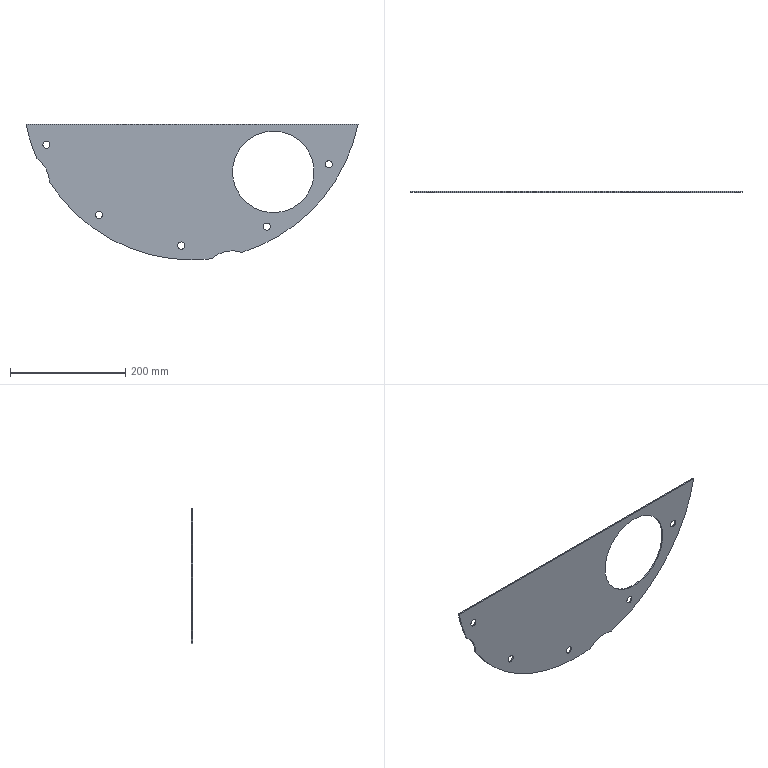Part | SolidWorks | features BaseBody 1 | 1 solid | 22 faces | box 577 x 2 x 236 mm | volume 170029 mm3 | cylinder 19 | plane 3 | commonest cylinder face diameters 12.5 x10 588.679 x4 106 x3 142 x2
STEP:
#1=CARTESIAN_POINT('',(237.632,2.,-121.934));
#2=VERTEX_POINT('',#1);
#3=CARTESIAN_POINT('',(237.632,2.,-134.434));
#4=VERTEX_POINT('',#3);
#5=CARTESIAN_POINT('',(237.632,2.,-128.184));
#6=DIRECTION('',(0.,-1.,0.));
#7=DIRECTION('',(0.,0.,-1.));
#8=AXIS2_PLACEMENT_3D('',#5,#6,#7);
#9=CIRCLE('',#8,6.25);
#10=EDGE_CURVE('',#2,#4,#9,.T.);
#11=ORIENTED_EDGE('',*,*,#10,.F.);
#12=CARTESIAN_POINT('',(237.632,0.,-121.934));
#13=VERTEX_POINT('',#12);
#14=CARTESIAN_POINT('',(237.632,2.,-121.934));
#15=DIRECTION('',(0.,-1.,0.));
#16=VECTOR('',#15,1000.);
#17=LINE('',#14,#16);
#18=EDGE_CURVE('',#2,#13,#17,.T.);
#19=ORIENTED_EDGE('',*,*,#18,.T.);
#20=CARTESIAN_POINT('',(237.632,0.,-134.434));
#21=VERTEX_POINT('',#20);
#22=CARTESIAN_POINT('',(237.632,0.,-128.184));
#23=DIRECTION('',(0.,1.,0.));
#24=DIRECTION('',(0.,0.,-1.));
#25=AXIS2_PLACEMENT_3D('',#22,#23,#24);
#26=CIRCLE('',#25,6.25);
#27=EDGE_CURVE('',#21,#13,#26,.T.);
#28=ORIENTED_EDGE('',*,*,#27,.F.);
#29=CARTESIAN_POINT('',(237.632,2.,-134.434));
#30=DIRECTION('',(0.,-1.,0.));
#31=VECTOR('',#30,1000.);
#32=LINE('',#29,#31);
#33=EDGE_CURVE('',#4,#21,#32,.T.);
#34=ORIENTED_EDGE('',*,*,#33,.F.);
#35=EDGE_LOOP('',(#11,#19,#28,#34));
#36=FACE_OUTER_BOUND('',#35,.T.);
#37=CARTESIAN_POINT('',(237.632,2.,-128.184));
#38=DIRECTION('',(0.,-1.,0.));
#39=DIRECTION('',(0.,0.,-1.));
#40=AXIS2_PLACEMENT_3D('',#37,#38,#39);
#41=CYLINDRICAL_SURFACE('',#40,6.25);
#42=ADVANCED_FACE('',(#36),#41,.F.);
#43=CARTESIAN_POINT('',(-18.702,2.,-263.101));
#44=VERTEX_POINT('',#43);
#45=CARTESIAN_POINT('',(-18.702,2.,-275.601));
#46=VERTEX_POINT('',#45);
#47=CARTESIAN_POINT('',(-18.702,2.,-269.351));
#48=DIRECTION('',(0.,-1.,0.));
#49=DIRECTION('',(0.,0.,-1.));
#50=AXIS2_PLACEMENT_3D('',#47,#48,#49);
#51=CIRCLE('',#50,6.25);
#52=EDGE_CURVE('',#44,#46,#51,.T.);
#53=ORIENTED_EDGE('',*,*,#52,.F.);
#54=CARTESIAN_POINT('',(-18.702,0.,-263.101));
#55=VERTEX_POINT('',#54);
#56=CARTESIAN_POINT('',(-18.702,2.,-263.101));
#57=DIRECTION('',(0.,-1.,0.));
#58=VECTOR('',#57,1000.);
#59=LINE('',#56,#58);
#60=EDGE_CURVE('',#44,#55,#59,.T.);
#61=ORIENTED_EDGE('',*,*,#60,.T.);
#62=CARTESIAN_POINT('',(-18.702,0.,-275.601));
#63=VERTEX_POINT('',#62);
#64=CARTESIAN_POINT('',(-18.702,0.,-269.351));
#65=DIRECTION('',(0.,1.,0.));
#66=DIRECTION('',(0.,0.,-1.));
#67=AXIS2_PLACEMENT_3D('',#64,#65,#66);
#68=CIRCLE('',#67,6.25);
#69=EDGE_CURVE('',#63,#55,#68,.T.);
#70=ORIENTED_EDGE('',*,*,#69,.F.);
#71=CARTESIAN_POINT('',(-18.702,2.,-275.601));
#72=DIRECTION('',(0.,-1.,0.));
#73=VECTOR('',#72,1000.);
#74=LINE('',#71,#73);
#75=EDGE_CURVE('',#46,#63,#74,.T.);
#76=ORIENTED_EDGE('',*,*,#75,.F.);
#77=EDGE_LOOP('',(#53,#61,#70,#76));
#78=FACE_OUTER_BOUND('',#77,.T.);
#79=CARTESIAN_POINT('',(-18.702,2.,-269.351));
#80=DIRECTION('',(0.,-1.,0.));
#81=DIRECTION('',(0.,0.,-1.));
#82=AXIS2_PLACEMENT_3D('',#79,#80,#81);
#83=CYLINDRICAL_SURFACE('',#82,6.25);
#84=ADVANCED_FACE('',(#78),#83,.F.);
#85=CARTESIAN_POINT('',(-253.067,2.,-87.863));
#86=VERTEX_POINT('',#85);
#87=CARTESIAN_POINT('',(-253.067,2.,-100.363));
#88=VERTEX_POINT('',#87);
#89=CARTESIAN_POINT('',(-253.067,2.,-94.113));
#90=DIRECTION('',(0.,-1.,0.));
#91=DIRECTION('',(0.,0.,-1.));
#92=AXIS2_PLACEMENT_3D('',#89,#90,#91);
#93=CIRCLE('',#92,6.25);
#94=EDGE_CURVE('',#86,#88,#93,.T.);
#95=ORIENTED_EDGE('',*,*,#94,.F.);
#96=CARTESIAN_POINT('',(-253.067,0.,-87.863));
#97=VERTEX_POINT('',#96);
#98=CARTESIAN_POINT('',(-253.067,2.,-87.863));
#99=DIRECTION('',(0.,-1.,0.));
#100=VECTOR('',#99,1000.);
#101=LINE('',#98,#100);
#102=EDGE_CURVE('',#86,#97,#101,.T.);
#103=ORIENTED_EDGE('',*,*,#102,.T.);
#104=CARTESIAN_POINT('',(-253.067,0.,-100.363));
#105=VERTEX_POINT('',#104);
#106=CARTESIAN_POINT('',(-253.067,0.,-94.113));
#107=DIRECTION('',(0.,1.,0.));
#108=DIRECTION('',(0.,0.,-1.));
#109=AXIS2_PLACEMENT_3D('',#106,#107,#108);
#110=CIRCLE('',#109,6.25);
#111=EDGE_CURVE('',#105,#97,#110,.T.);
#112=ORIENTED_EDGE('',*,*,#111,.F.);
#113=CARTESIAN_POINT('',(-253.067,2.,-100.363));
#114=DIRECTION('',(0.,-1.,0.));
#115=VECTOR('',#114,1000.);
#116=LINE('',#113,#115);
#117=EDGE_CURVE('',#88,#105,#116,.T.);
#118=ORIENTED_EDGE('',*,*,#117,.F.);
#119=EDGE_LOOP('',(#95,#103,#112,#118));
#120=FACE_OUTER_BOUND('',#119,.T.);
#121=CARTESIAN_POINT('',(-253.067,2.,-94.113));
#122=DIRECTION('',(0.,-1.,0.));
#123=DIRECTION('',(0.,0.,-1.));
#124=AXIS2_PLACEMENT_3D('',#121,#122,#123);
#125=CYLINDRICAL_SURFACE('',#124,6.25);
#126=ADVANCED_FACE('',(#120),#125,.F.);
#127=CARTESIAN_POINT('',(-161.684,2.,-209.987));
#128=VERTEX_POINT('',#127);
#129=CARTESIAN_POINT('',(-161.684,2.,-222.487));
#130=VERTEX_POINT('',#129);
#131=CARTESIAN_POINT('',(-161.684,2.,-216.237));
#132=DIRECTION('',(0.,-1.,0.));
#133=DIRECTION('',(0.,0.,-1.));
#134=AXIS2_PLACEMENT_3D('',#131,#132,#133);
#135=CIRCLE('',#134,6.25);
#136=EDGE_CURVE('',#128,#130,#135,.T.);
#137=ORIENTED_EDGE('',*,*,#136,.F.);
#138=CARTESIAN_POINT('',(-161.684,0.,-209.987));
#139=VERTEX_POINT('',#138);
#140=CARTESIAN_POINT('',(-161.684,2.,-209.987));
#141=DIRECTION('',(0.,-1.,0.));
#142=VECTOR('',#141,1000.);
#143=LINE('',#140,#142);
#144=EDGE_CURVE('',#128,#139,#143,.T.);
#145=ORIENTED_EDGE('',*,*,#144,.T.);
#146=CARTESIAN_POINT('',(-161.684,0.,-222.487));
#147=VERTEX_POINT('',#146);
#148=CARTESIAN_POINT('',(-161.684,0.,-216.237));
#149=DIRECTION('',(0.,1.,0.));
#150=DIRECTION('',(0.,0.,-1.));
#151=AXIS2_PLACEMENT_3D('',#148,#149,#150);
#152=CIRCLE('',#151,6.25);
#153=EDGE_CURVE('',#147,#139,#152,.T.);
#154=ORIENTED_EDGE('',*,*,#153,.F.);
#155=CARTESIAN_POINT('',(-161.684,2.,-222.487));
#156=DIRECTION('',(0.,-1.,0.));
#157=VECTOR('',#156,1000.);
#158=LINE('',#155,#157);
#159=EDGE_CURVE('',#130,#147,#158,.T.);
#160=ORIENTED_EDGE('',*,*,#159,.F.);
#161=EDGE_LOOP('',(#137,#145,#154,#160));
#162=FACE_OUTER_BOUND('',#161,.T.);
#163=CARTESIAN_POINT('',(-161.684,2.,-216.237));
#164=DIRECTION('',(0.,-1.,0.));
#165=DIRECTION('',(0.,0.,-1.));
#166=AXIS2_PLACEMENT_3D('',#163,#164,#165);
#167=CYLINDRICAL_SURFACE('',#166,6.25);
#168=ADVANCED_FACE('',(#162),#167,.F.);
#169=CARTESIAN_POINT('',(130.248,2.,-230.257));
#170=VERTEX_POINT('',#169);
#171=CARTESIAN_POINT('',(130.248,2.,-242.757));
#172=VERTEX_POINT('',#171);
#173=CARTESIAN_POINT('',(130.248,2.,-236.507));
#174=DIRECTION('',(0.,-1.,0.));
#175=DIRECTION('',(0.,0.,-1.));
#176=AXIS2_PLACEMENT_3D('',#173,#174,#175);
#177=CIRCLE('',#176,6.25);
#178=EDGE_CURVE('',#170,#172,#177,.T.);
#179=ORIENTED_EDGE('',*,*,#178,.F.);
#180=CARTESIAN_POINT('',(130.248,0.,-230.257));
#181=VERTEX_POINT('',#180);
#182=CARTESIAN_POINT('',(130.248,2.,-230.257));
#183=DIRECTION('',(0.,-1.,0.));
#184=VECTOR('',#183,1000.);
#185=LINE('',#182,#184);
#186=EDGE_CURVE('',#170,#181,#185,.T.);
#187=ORIENTED_EDGE('',*,*,#186,.T.);
#188=CARTESIAN_POINT('',(130.248,0.,-242.757));
#189=VERTEX_POINT('',#188);
#190=CARTESIAN_POINT('',(130.248,0.,-236.507));
#191=DIRECTION('',(0.,1.,0.));
#192=DIRECTION('',(0.,0.,-1.));
#193=AXIS2_PLACEMENT_3D('',#190,#191,#192);
#194=CIRCLE('',#193,6.25);
#195=EDGE_CURVE('',#189,#181,#194,.T.);
#196=ORIENTED_EDGE('',*,*,#195,.F.);
#197=CARTESIAN_POINT('',(130.248,2.,-242.757));
#198=DIRECTION('',(0.,-1.,0.));
#199=VECTOR('',#198,1000.);
#200=LINE('',#197,#199);
#201=EDGE_CURVE('',#172,#189,#200,.T.);
#202=ORIENTED_EDGE('',*,*,#201,.F.);
#203=EDGE_LOOP('',(#179,#187,#196,#202));
#204=FACE_OUTER_BOUND('',#203,.T.);
#205=CARTESIAN_POINT('',(130.248,2.,-236.507));
#206=DIRECTION('',(0.,-1.,0.));
#207=DIRECTION('',(0.,0.,-1.));
#208=AXIS2_PLACEMENT_3D('',#205,#206,#207);
#209=CYLINDRICAL_SURFACE('',#208,6.25);
#210=ADVANCED_FACE('',(#204),#209,.F.);
#211=CARTESIAN_POINT('',(69.671,0.,-278.59));
#212=VERTEX_POINT('',#211);
#213=CARTESIAN_POINT('',(86.515,0.,-281.338));
#214=VERTEX_POINT('',#213);
#215=CARTESIAN_POINT('',(69.671,0.,-331.59));
#216=DIRECTION('',(0.,1.,0.));
#217=DIRECTION('',(0.,0.,1.));
#218=AXIS2_PLACEMENT_3D('',#215,#216,#217);
#219=CIRCLE('',#218,53.);
#220=EDGE_CURVE('',#212,#214,#219,.T.);
#221=ORIENTED_EDGE('',*,*,#220,.F.);
#222=CARTESIAN_POINT('',(69.671,2.,-278.59));
#223=VERTEX_POINT('',#222);
#224=CARTESIAN_POINT('',(69.671,-8.,-278.59));
#225=DIRECTION('',(0.,1.,0.));
#226=VECTOR('',#225,1000.);
#227=LINE('',#224,#226);
#228=EDGE_CURVE('',#212,#223,#227,.T.);
#229=ORIENTED_EDGE('',*,*,#228,.T.);
#230=CARTESIAN_POINT('',(86.515,2.,-281.338));
#231=VERTEX_POINT('',#230);
#232=CARTESIAN_POINT('',(69.671,2.,-331.59));
#233=DIRECTION('',(0.,-1.,0.));
#234=DIRECTION('',(0.,0.,1.));
#235=AXIS2_PLACEMENT_3D('',#232,#233,#234);
#236=CIRCLE('',#235,53.);
#237=EDGE_CURVE('',#231,#223,#236,.T.);
#238=ORIENTED_EDGE('',*,*,#237,.F.);
#239=CARTESIAN_POINT('',(86.515,-8.,-281.338));
#240=DIRECTION('',(0.,1.,0.));
#241=VECTOR('',#240,1000.);
#242=LINE('',#239,#241);
#243=EDGE_CURVE('',#214,#231,#242,.T.);
#244=ORIENTED_EDGE('',*,*,#243,.F.);
#245=EDGE_LOOP('',(#221,#229,#238,#244));
#246=FACE_OUTER_BOUND('',#245,.T.);
#247=CARTESIAN_POINT('',(69.671,-8.,-331.59));
#248=DIRECTION('',(0.,1.,0.));
#249=DIRECTION('',(0.,0.,1.));
#250=AXIS2_PLACEMENT_3D('',#247,#248,#249);
#251=CYLINDRICAL_SURFACE('',#250,53.);
#252=ADVANCED_FACE('',(#246),#251,.F.);
#253=CARTESIAN_POINT('',(0.,2.,-294.34));
#254=VERTEX_POINT('',#253);
#255=CARTESIAN_POINT('',(-247.369,2.,-159.512));
#256=VERTEX_POINT('',#255);
#257=CARTESIAN_POINT('',(0.,2.,0.));
#258=DIRECTION('',(0.,1.,0.));
#259=DIRECTION('',(0.,0.,-1.));
#260=AXIS2_PLACEMENT_3D('',#257,#258,#259);
#261=CIRCLE('',#260,294.34);
#262=EDGE_CURVE('',#254,#256,#261,.T.);
#263=ORIENTED_EDGE('',*,*,#262,.F.);
#264=CARTESIAN_POINT('',(0.,0.,-294.34));
#265=VERTEX_POINT('',#264);
#266=CARTESIAN_POINT('',(0.,2.,-294.34));
#267=DIRECTION('',(0.,-1.,0.));
#268=VECTOR('',#267,1000.);
#269=LINE('',#266,#268);
#270=EDGE_CURVE('',#254,#265,#269,.T.);
#271=ORIENTED_EDGE('',*,*,#270,.T.);
#272=CARTESIAN_POINT('',(-247.369,0.,-159.512));
#273=VERTEX_POINT('',#272);
#274=CARTESIAN_POINT('',(0.,0.,0.));
#275=DIRECTION('',(0.,1.,0.));
#276=DIRECTION('',(0.,0.,-1.));
#277=AXIS2_PLACEMENT_3D('',#274,#275,#276);
#278=CIRCLE('',#277,294.34);
#279=EDGE_CURVE('',#265,#273,#278,.T.);
#280=ORIENTED_EDGE('',*,*,#279,.T.);
#281=CARTESIAN_POINT('',(-247.369,-8.,-159.512));
#282=DIRECTION('',(0.,1.,0.));
#283=VECTOR('',#282,1000.);
#284=LINE('',#281,#283);
#285=EDGE_CURVE('',#273,#256,#284,.T.);
#286=ORIENTED_EDGE('',*,*,#285,.T.);
#287=EDGE_LOOP('',(#263,#271,#280,#286));
#288=FACE_OUTER_BOUND('',#287,.T.);
#289=CARTESIAN_POINT('',(0.,2.,0.));
#290=DIRECTION('',(0.,-1.,0.));
#291=DIRECTION('',(0.,0.,-1.));
#292=AXIS2_PLACEMENT_3D('',#289,#290,#291);
#293=CYLINDRICAL_SURFACE('',#292,294.34);
#294=ADVANCED_FACE('',(#288),#293,.T.);
#295=CARTESIAN_POINT('',(141.421,0.,-212.421));
#296=VERTEX_POINT('',#295);
#297=CARTESIAN_POINT('',(141.421,0.,-70.421));
#298=VERTEX_POINT('',#297);
#299=CARTESIAN_POINT('',(141.421,0.,-141.421));
#300=DIRECTION('',(0.,1.,0.));
#301=DIRECTION('',(0.,0.,1.));
#302=AXIS2_PLACEMENT_3D('',#299,#300,#301);
#303=CIRCLE('',#302,71.);
#304=EDGE_CURVE('',#296,#298,#303,.T.);
#305=ORIENTED_EDGE('',*,*,#304,.F.);
#306=CARTESIAN_POINT('',(141.421,2.,-212.421));
#307=VERTEX_POINT('',#306);
#308=CARTESIAN_POINT('',(141.421,-8.,-212.421));
#309=DIRECTION('',(0.,1.,0.));
#310=VECTOR('',#309,1000.);
#311=LINE('',#308,#310);
#312=EDGE_CURVE('',#296,#307,#311,.T.);
#313=ORIENTED_EDGE('',*,*,#312,.T.);
#314=CARTESIAN_POINT('',(141.421,2.,-70.421));
#315=VERTEX_POINT('',#314);
#316=CARTESIAN_POINT('',(141.421,2.,-141.421));
#317=DIRECTION('',(0.,-1.,0.));
#318=DIRECTION('',(0.,0.,1.));
#319=AXIS2_PLACEMENT_3D('',#316,#317,#318);
#320=CIRCLE('',#319,71.);
#321=EDGE_CURVE('',#315,#307,#320,.T.);
#322=ORIENTED_EDGE('',*,*,#321,.F.);
#323=CARTESIAN_POINT('',(141.421,-8.,-70.421));
#324=DIRECTION('',(0.,1.,0.));
#325=VECTOR('',#324,1000.);
#326=LINE('',#323,#325);
#327=EDGE_CURVE('',#298,#315,#326,.T.);
#328=ORIENTED_EDGE('',*,*,#327,.F.);
#329=EDGE_LOOP('',(#305,#313,#322,#328));
#330=FACE_OUTER_BOUND('',#329,.T.);
#331=CARTESIAN_POINT('',(141.421,-8.,-141.421));
#332=DIRECTION('',(0.,1.,0.));
#333=DIRECTION('',(0.,0.,1.));
#334=AXIS2_PLACEMENT_3D('',#331,#332,#333);
#335=CYLINDRICAL_SURFACE('',#334,71.);
#336=ADVANCED_FACE('',(#330),#335,.F.);
#337=CARTESIAN_POINT('',(237.632,2.,-128.184));
#338=DIRECTION('',(0.,-1.,0.));
#339=DIRECTION('',(0.,0.,-1.));
#340=AXIS2_PLACEMENT_3D('',#337,#338,#339);
#341=CIRCLE('',#340,6.25);
#342=EDGE_CURVE('',#4,#2,#341,.T.);
#343=ORIENTED_EDGE('',*,*,#342,.T.);
#344=ORIENTED_EDGE('',*,*,#10,.T.);
#345=EDGE_LOOP('',(#343,#344));
#346=FACE_BOUND('',#345,.T.);
#347=CARTESIAN_POINT('',(-18.702,2.,-269.351));
#348=DIRECTION('',(0.,-1.,0.));
#349=DIRECTION('',(0.,0.,-1.));
#350=AXIS2_PLACEMENT_3D('',#347,#348,#349);
#351=CIRCLE('',#350,6.25);
#352=EDGE_CURVE('',#46,#44,#351,.T.);
#353=ORIENTED_EDGE('',*,*,#352,.T.);
#354=ORIENTED_EDGE('',*,*,#52,.T.);
#355=EDGE_LOOP('',(#353,#354));
#356=FACE_BOUND('',#355,.T.);
#357=CARTESIAN_POINT('',(-253.067,2.,-94.113));
#358=DIRECTION('',(0.,-1.,0.));
#359=DIRECTION('',(0.,0.,-1.));
#360=AXIS2_PLACEMENT_3D('',#357,#358,#359);
#361=CIRCLE('',#360,6.25);
#362=EDGE_CURVE('',#88,#86,#361,.T.);
#363=ORIENTED_EDGE('',*,*,#362,.T.);
#364=ORIENTED_EDGE('',*,*,#94,.T.);
#365=EDGE_LOOP('',(#363,#364));
#366=FACE_BOUND('',#365,.T.);
#367=CARTESIAN_POINT('',(-161.684,2.,-216.237));
#368=DIRECTION('',(0.,-1.,0.));
#369=DIRECTION('',(0.,0.,-1.));
#370=AXIS2_PLACEMENT_3D('',#367,#368,#369);
#371=CIRCLE('',#370,6.25);
#372=EDGE_CURVE('',#130,#128,#371,.T.);
#373=ORIENTED_EDGE('',*,*,#372,.T.);
#374=ORIENTED_EDGE('',*,*,#136,.T.);
#375=EDGE_LOOP('',(#373,#374));
#376=FACE_BOUND('',#375,.T.);
#377=CARTESIAN_POINT('',(130.248,2.,-236.507));
#378=DIRECTION('',(0.,-1.,0.));
#379=DIRECTION('',(0.,0.,-1.));
#380=AXIS2_PLACEMENT_3D('',#377,#378,#379);
#381=CIRCLE('',#380,6.25);
#382=EDGE_CURVE('',#172,#170,#381,.T.);
#383=ORIENTED_EDGE('',*,*,#382,.T.);
#384=ORIENTED_EDGE('',*,*,#178,.T.);
#385=EDGE_LOOP('',(#383,#384));
#386=FACE_BOUND('',#385,.T.);
#387=CARTESIAN_POINT('',(288.5,2.,-58.34));
#388=VERTEX_POINT('',#387);
#389=CARTESIAN_POINT('',(0.,2.,0.));
#390=DIRECTION('',(0.,1.,0.));
#391=DIRECTION('',(0.,0.,-1.));
#392=AXIS2_PLACEMENT_3D('',#389,#390,#391);
#393=CIRCLE('',#392,294.34);
#394=EDGE_CURVE('',#388,#231,#393,.T.);
#395=ORIENTED_EDGE('',*,*,#394,.T.);
#396=ORIENTED_EDGE('',*,*,#237,.T.);
#397=CARTESIAN_POINT('',(34.027,2.,-292.366));
#398=VERTEX_POINT('',#397);
#399=CARTESIAN_POINT('',(69.671,2.,-331.59));
#400=DIRECTION('',(0.,-1.,0.));
#401=DIRECTION('',(0.,0.,1.));
#402=AXIS2_PLACEMENT_3D('',#399,#400,#401);
#403=CIRCLE('',#402,53.);
#404=EDGE_CURVE('',#223,#398,#403,.T.);
#405=ORIENTED_EDGE('',*,*,#404,.T.);
#406=CARTESIAN_POINT('',(0.,2.,0.));
#407=DIRECTION('',(0.,1.,0.));
#408=DIRECTION('',(0.,0.,-1.));
#409=AXIS2_PLACEMENT_3D('',#406,#407,#408);
#410=CIRCLE('',#409,294.34);
#411=EDGE_CURVE('',#398,#254,#410,.T.);
#412=ORIENTED_EDGE('',*,*,#411,.T.);
#413=ORIENTED_EDGE('',*,*,#262,.T.);
#414=CARTESIAN_POINT('',(-269.414,2.,-118.54));
#415=VERTEX_POINT('',#414);
#416=CARTESIAN_POINT('',(-300.329,2.,-161.59));
#417=DIRECTION('',(0.,-1.,0.));
#418=DIRECTION('',(0.,0.,1.));
#419=AXIS2_PLACEMENT_3D('',#416,#417,#418);
#420=CIRCLE('',#419,53.);
#421=EDGE_CURVE('',#256,#415,#420,.T.);
#422=ORIENTED_EDGE('',*,*,#421,.T.);
#423=CARTESIAN_POINT('',(-288.5,2.,-58.34));
#424=VERTEX_POINT('',#423);
#425=CARTESIAN_POINT('',(0.,2.,0.));
#426=DIRECTION('',(0.,1.,0.));
#427=DIRECTION('',(0.,0.,-1.));
#428=AXIS2_PLACEMENT_3D('',#425,#426,#427);
#429=CIRCLE('',#428,294.34);
#430=EDGE_CURVE('',#415,#424,#429,.T.);
#431=ORIENTED_EDGE('',*,*,#430,.T.);
#432=CARTESIAN_POINT('',(0.,2.,-58.34));
#433=DIRECTION('',(1.,0.,0.));
#434=VECTOR('',#433,1000.);
#435=LINE('',#432,#434);
#436=EDGE_CURVE('',#424,#388,#435,.T.);
#437=ORIENTED_EDGE('',*,*,#436,.T.);
#438=EDGE_LOOP('',(#395,#396,#405,#412,#413,#422,#431,#437));
#439=FACE_OUTER_BOUND('',#438,.T.);
#440=ORIENTED_EDGE('',*,*,#321,.T.);
#441=CARTESIAN_POINT('',(141.421,2.,-141.421));
#442=DIRECTION('',(0.,-1.,0.));
#443=DIRECTION('',(0.,0.,1.));
#444=AXIS2_PLACEMENT_3D('',#441,#442,#443);
#445=CIRCLE('',#444,71.);
#446=EDGE_CURVE('',#307,#315,#445,.T.);
#447=ORIENTED_EDGE('',*,*,#446,.T.);
#448=EDGE_LOOP('',(#440,#447));
#449=FACE_BOUND('',#448,.T.);
#450=CARTESIAN_POINT('',(0.,2.,0.));
#451=DIRECTION('',(0.,1.,0.));
#452=DIRECTION('',(0.,0.,1.));
#453=AXIS2_PLACEMENT_3D('',#450,#451,#452);
#454=PLANE('',#453);
#455=ADVANCED_FACE('',(#346,#356,#366,#376,#386,#439,#449),#454,.T.);
#456=ORIENTED_EDGE('',*,*,#18,.F.);
#457=ORIENTED_EDGE('',*,*,#342,.F.);
#458=ORIENTED_EDGE('',*,*,#33,.T.);
#459=CARTESIAN_POINT('',(237.632,0.,-128.184));
#460=DIRECTION('',(0.,1.,0.));
#461=DIRECTION('',(0.,0.,-1.));
#462=AXIS2_PLACEMENT_3D('',#459,#460,#461);
#463=CIRCLE('',#462,6.25);
#464=EDGE_CURVE('',#13,#21,#463,.T.);
#465=ORIENTED_EDGE('',*,*,#464,.F.);
#466=EDGE_LOOP('',(#456,#457,#458,#465));
#467=FACE_OUTER_BOUND('',#466,.T.);
#468=CARTESIAN_POINT('',(237.632,2.,-128.184));
#469=DIRECTION('',(0.,-1.,0.));
#470=DIRECTION('',(0.,0.,-1.));
#471=AXIS2_PLACEMENT_3D('',#468,#469,#470);
#472=CYLINDRICAL_SURFACE('',#471,6.25);
#473=ADVANCED_FACE('',(#467),#472,.F.);
#474=ORIENTED_EDGE('',*,*,#60,.F.);
#475=ORIENTED_EDGE('',*,*,#352,.F.);
#476=ORIENTED_EDGE('',*,*,#75,.T.);
#477=CARTESIAN_POINT('',(-18.702,0.,-269.351));
#478=DIRECTION('',(0.,1.,0.));
#479=DIRECTION('',(0.,0.,-1.));
#480=AXIS2_PLACEMENT_3D('',#477,#478,#479);
#481=CIRCLE('',#480,6.25);
#482=EDGE_CURVE('',#55,#63,#481,.T.);
#483=ORIENTED_EDGE('',*,*,#482,.F.);
#484=EDGE_LOOP('',(#474,#475,#476,#483));
#485=FACE_OUTER_BOUND('',#484,.T.);
#486=CARTESIAN_POINT('',(-18.702,2.,-269.351));
#487=DIRECTION('',(0.,-1.,0.));
#488=DIRECTION('',(0.,0.,-1.));
#489=AXIS2_PLACEMENT_3D('',#486,#487,#488);
#490=CYLINDRICAL_SURFACE('',#489,6.25);
#491=ADVANCED_FACE('',(#485),#490,.F.);
#492=ORIENTED_EDGE('',*,*,#102,.F.);
#493=ORIENTED_EDGE('',*,*,#362,.F.);
#494=ORIENTED_EDGE('',*,*,#117,.T.);
#495=CARTESIAN_POINT('',(-253.067,0.,-94.113));
#496=DIRECTION('',(0.,1.,0.));
#497=DIRECTION('',(0.,0.,-1.));
#498=AXIS2_PLACEMENT_3D('',#495,#496,#497);
#499=CIRCLE('',#498,6.25);
#500=EDGE_CURVE('',#97,#105,#499,.T.);
#501=ORIENTED_EDGE('',*,*,#500,.F.);
#502=EDGE_LOOP('',(#492,#493,#494,#501));
#503=FACE_OUTER_BOUND('',#502,.T.);
#504=CARTESIAN_POINT('',(-253.067,2.,-94.113));
#505=DIRECTION('',(0.,-1.,0.));
#506=DIRECTION('',(0.,0.,-1.));
#507=AXIS2_PLACEMENT_3D('',#504,#505,#506);
#508=CYLINDRICAL_SURFACE('',#507,6.25);
#509=ADVANCED_FACE('',(#503),#508,.F.);
#510=ORIENTED_EDGE('',*,*,#144,.F.);
#511=ORIENTED_EDGE('',*,*,#372,.F.);
#512=ORIENTED_EDGE('',*,*,#159,.T.);
#513=CARTESIAN_POINT('',(-161.684,0.,-216.237));
#514=DIRECTION('',(0.,1.,0.));
#515=DIRECTION('',(0.,0.,-1.));
#516=AXIS2_PLACEMENT_3D('',#513,#514,#515);
#517=CIRCLE('',#516,6.25);
#518=EDGE_CURVE('',#139,#147,#517,.T.);
#519=ORIENTED_EDGE('',*,*,#518,.F.);
#520=EDGE_LOOP('',(#510,#511,#512,#519));
#521=FACE_OUTER_BOUND('',#520,.T.);
#522=CARTESIAN_POINT('',(-161.684,2.,-216.237));
#523=DIRECTION('',(0.,-1.,0.));
#524=DIRECTION('',(0.,0.,-1.));
#525=AXIS2_PLACEMENT_3D('',#522,#523,#524);
#526=CYLINDRICAL_SURFACE('',#525,6.25);
#527=ADVANCED_FACE('',(#521),#526,.F.);
#528=ORIENTED_EDGE('',*,*,#186,.F.);
#529=ORIENTED_EDGE('',*,*,#382,.F.);
#530=ORIENTED_EDGE('',*,*,#201,.T.);
#531=CARTESIAN_POINT('',(130.248,0.,-236.507));
#532=DIRECTION('',(0.,1.,0.));
#533=DIRECTION('',(0.,0.,-1.));
#534=AXIS2_PLACEMENT_3D('',#531,#532,#533);
#535=CIRCLE('',#534,6.25);
#536=EDGE_CURVE('',#181,#189,#535,.T.);
#537=ORIENTED_EDGE('',*,*,#536,.F.);
#538=EDGE_LOOP('',(#528,#529,#530,#537));
#539=FACE_OUTER_BOUND('',#538,.T.);
#540=CARTESIAN_POINT('',(130.248,2.,-236.507));
#541=DIRECTION('',(0.,-1.,0.));
#542=DIRECTION('',(0.,0.,-1.));
#543=AXIS2_PLACEMENT_3D('',#540,#541,#542);
#544=CYLINDRICAL_SURFACE('',#543,6.25);
#545=ADVANCED_FACE('',(#539),#544,.F.);
#546=ORIENTED_EDGE('',*,*,#228,.F.);
#547=CARTESIAN_POINT('',(34.027,0.,-292.366));
#548=VERTEX_POINT('',#547);
#549=CARTESIAN_POINT('',(69.671,0.,-331.59));
#550=DIRECTION('',(0.,1.,0.));
#551=DIRECTION('',(0.,0.,1.));
#552=AXIS2_PLACEMENT_3D('',#549,#550,#551);
#553=CIRCLE('',#552,53.);
#554=EDGE_CURVE('',#548,#212,#553,.T.);
#555=ORIENTED_EDGE('',*,*,#554,.F.);
#556=CARTESIAN_POINT('',(34.027,2.,-292.366));
#557=DIRECTION('',(0.,-1.,0.));
#558=VECTOR('',#557,1000.);
#559=LINE('',#556,#558);
#560=EDGE_CURVE('',#398,#548,#559,.T.);
#561=ORIENTED_EDGE('',*,*,#560,.F.);
#562=ORIENTED_EDGE('',*,*,#404,.F.);
#563=EDGE_LOOP('',(#546,#555,#561,#562));
#564=FACE_OUTER_BOUND('',#563,.T.);
#565=CARTESIAN_POINT('',(69.671,-8.,-331.59));
#566=DIRECTION('',(0.,1.,0.));
#567=DIRECTION('',(0.,0.,1.));
#568=AXIS2_PLACEMENT_3D('',#565,#566,#567);
#569=CYLINDRICAL_SURFACE('',#568,53.);
#570=ADVANCED_FACE('',(#564),#569,.F.);
#571=ORIENTED_EDGE('',*,*,#394,.F.);
#572=CARTESIAN_POINT('',(288.5,0.,-58.34));
#573=VERTEX_POINT('',#572);
#574=CARTESIAN_POINT('',(288.5,2.,-58.34));
#575=DIRECTION('',(0.,-1.,0.));
#576=VECTOR('',#575,1000.);
#577=LINE('',#574,#576);
#578=EDGE_CURVE('',#388,#573,#577,.T.);
#579=ORIENTED_EDGE('',*,*,#578,.T.);
#580=CARTESIAN_POINT('',(0.,0.,0.));
#581=DIRECTION('',(0.,1.,0.));
#582=DIRECTION('',(0.,0.,-1.));
#583=AXIS2_PLACEMENT_3D('',#580,#581,#582);
#584=CIRCLE('',#583,294.34);
#585=EDGE_CURVE('',#573,#214,#584,.T.);
#586=ORIENTED_EDGE('',*,*,#585,.T.);
#587=ORIENTED_EDGE('',*,*,#243,.T.);
#588=EDGE_LOOP('',(#571,#579,#586,#587));
#589=FACE_OUTER_BOUND('',#588,.T.);
#590=CARTESIAN_POINT('',(0.,2.,0.));
#591=DIRECTION('',(0.,-1.,0.));
#592=DIRECTION('',(0.,0.,-1.));
#593=AXIS2_PLACEMENT_3D('',#590,#591,#592);
#594=CYLINDRICAL_SURFACE('',#593,294.34);
#595=ADVANCED_FACE('',(#589),#594,.T.);
#596=ORIENTED_EDGE('',*,*,#578,.F.);
#597=ORIENTED_EDGE('',*,*,#436,.F.);
#598=CARTESIAN_POINT('',(-288.5,0.,-58.34));
#599=VERTEX_POINT('',#598);
#600=CARTESIAN_POINT('',(-288.5,2.,-58.34));
#601=DIRECTION('',(0.,1.,0.));
#602=VECTOR('',#601,1000.);
#603=LINE('',#600,#602);
#604=EDGE_CURVE('',#599,#424,#603,.T.);
#605=ORIENTED_EDGE('',*,*,#604,.F.);
#606=CARTESIAN_POINT('',(-288.5,0.,-58.34));
#607=DIRECTION('',(-1.,0.,0.));
#608=VECTOR('',#607,1000.);
#609=LINE('',#606,#608);
#610=EDGE_CURVE('',#573,#599,#609,.T.);
#611=ORIENTED_EDGE('',*,*,#610,.F.);
#612=EDGE_LOOP('',(#596,#597,#605,#611));
#613=FACE_OUTER_BOUND('',#612,.T.);
#614=CARTESIAN_POINT('',(-288.5,2.,-58.34));
#615=DIRECTION('',(0.,0.,-1.));
#616=DIRECTION('',(-1.,0.,0.));
#617=AXIS2_PLACEMENT_3D('',#614,#615,#616);
#618=PLANE('',#617);
#619=ADVANCED_FACE('',(#613),#618,.F.);
#620=CARTESIAN_POINT('',(-269.414,0.,-118.54));
#621=VERTEX_POINT('',#620);
#622=CARTESIAN_POINT('',(0.,0.,0.));
#623=DIRECTION('',(0.,1.,0.));
#624=DIRECTION('',(0.,0.,-1.));
#625=AXIS2_PLACEMENT_3D('',#622,#623,#624);
#626=CIRCLE('',#625,294.34);
#627=EDGE_CURVE('',#621,#599,#626,.T.);
#628=ORIENTED_EDGE('',*,*,#627,.T.);
#629=ORIENTED_EDGE('',*,*,#604,.T.);
#630=ORIENTED_EDGE('',*,*,#430,.F.);
#631=CARTESIAN_POINT('',(-269.414,2.,-118.54));
#632=DIRECTION('',(0.,-1.,0.));
#633=VECTOR('',#632,1000.);
#634=LINE('',#631,#633);
#635=EDGE_CURVE('',#415,#621,#634,.T.);
#636=ORIENTED_EDGE('',*,*,#635,.T.);
#637=EDGE_LOOP('',(#628,#629,#630,#636));
#638=FACE_OUTER_BOUND('',#637,.T.);
#639=CARTESIAN_POINT('',(0.,2.,0.));
#640=DIRECTION('',(0.,-1.,0.));
#641=DIRECTION('',(0.,0.,-1.));
#642=AXIS2_PLACEMENT_3D('',#639,#640,#641);
#643=CYLINDRICAL_SURFACE('',#642,294.34);
#644=ADVANCED_FACE('',(#638),#643,.T.);
#645=ORIENTED_EDGE('',*,*,#635,.F.);
#646=ORIENTED_EDGE('',*,*,#421,.F.);
#647=ORIENTED_EDGE('',*,*,#285,.F.);
#648=CARTESIAN_POINT('',(-300.329,0.,-161.59));
#649=DIRECTION('',(0.,1.,0.));
#650=DIRECTION('',(0.,0.,1.));
#651=AXIS2_PLACEMENT_3D('',#648,#649,#650);
#652=CIRCLE('',#651,53.);
#653=EDGE_CURVE('',#621,#273,#652,.T.);
#654=ORIENTED_EDGE('',*,*,#653,.F.);
#655=EDGE_LOOP('',(#645,#646,#647,#654));
#656=FACE_OUTER_BOUND('',#655,.T.);
#657=CARTESIAN_POINT('',(-300.329,-8.,-161.59));
#658=DIRECTION('',(0.,1.,0.));
#659=DIRECTION('',(0.,0.,1.));
#660=AXIS2_PLACEMENT_3D('',#657,#658,#659);
#661=CYLINDRICAL_SURFACE('',#660,53.);
#662=ADVANCED_FACE('',(#656),#661,.F.);
#663=ORIENTED_EDGE('',*,*,#270,.F.);
#664=ORIENTED_EDGE('',*,*,#411,.F.);
#665=ORIENTED_EDGE('',*,*,#560,.T.);
#666=CARTESIAN_POINT('',(0.,0.,0.));
#667=DIRECTION('',(0.,1.,0.));
#668=DIRECTION('',(0.,0.,-1.));
#669=AXIS2_PLACEMENT_3D('',#666,#667,#668);
#670=CIRCLE('',#669,294.34);
#671=EDGE_CURVE('',#548,#265,#670,.T.);
#672=ORIENTED_EDGE('',*,*,#671,.T.);
#673=EDGE_LOOP('',(#663,#664,#665,#672));
#674=FACE_OUTER_BOUND('',#673,.T.);
#675=CARTESIAN_POINT('',(0.,2.,0.));
#676=DIRECTION('',(0.,-1.,0.));
#677=DIRECTION('',(0.,0.,-1.));
#678=AXIS2_PLACEMENT_3D('',#675,#676,#677);
#679=CYLINDRICAL_SURFACE('',#678,294.34);
#680=ADVANCED_FACE('',(#674),#679,.T.);
#681=ORIENTED_EDGE('',*,*,#312,.F.);
#682=CARTESIAN_POINT('',(141.421,0.,-141.421));
#683=DIRECTION('',(0.,1.,0.));
#684=DIRECTION('',(0.,0.,1.));
#685=AXIS2_PLACEMENT_3D('',#682,#683,#684);
#686=CIRCLE('',#685,71.);
#687=EDGE_CURVE('',#298,#296,#686,.T.);
#688=ORIENTED_EDGE('',*,*,#687,.F.);
#689=ORIENTED_EDGE('',*,*,#327,.T.);
#690=ORIENTED_EDGE('',*,*,#446,.F.);
#691=EDGE_LOOP('',(#681,#688,#689,#690));
#692=FACE_OUTER_BOUND('',#691,.T.);
#693=CARTESIAN_POINT('',(141.421,-8.,-141.421));
#694=DIRECTION('',(0.,1.,0.));
#695=DIRECTION('',(0.,0.,1.));
#696=AXIS2_PLACEMENT_3D('',#693,#694,#695);
#697=CYLINDRICAL_SURFACE('',#696,71.);
#698=ADVANCED_FACE('',(#692),#697,.F.);
#699=ORIENTED_EDGE('',*,*,#27,.T.);
#700=ORIENTED_EDGE('',*,*,#464,.T.);
#701=EDGE_LOOP('',(#699,#700));
#702=FACE_BOUND('',#701,.T.);
#703=ORIENTED_EDGE('',*,*,#195,.T.);
#704=ORIENTED_EDGE('',*,*,#536,.T.);
#705=EDGE_LOOP('',(#703,#704));
#706=FACE_BOUND('',#705,.T.);
#707=ORIENTED_EDGE('',*,*,#69,.T.);
#708=ORIENTED_EDGE('',*,*,#482,.T.);
#709=EDGE_LOOP('',(#707,#708));
#710=FACE_BOUND('',#709,.T.);
#711=ORIENTED_EDGE('',*,*,#153,.T.);
#712=ORIENTED_EDGE('',*,*,#518,.T.);
#713=EDGE_LOOP('',(#711,#712));
#714=FACE_BOUND('',#713,.T.);
#715=ORIENTED_EDGE('',*,*,#111,.T.);
#716=ORIENTED_EDGE('',*,*,#500,.T.);
#717=EDGE_LOOP('',(#715,#716));
#718=FACE_BOUND('',#717,.T.);
#719=ORIENTED_EDGE('',*,*,#671,.F.);
#720=ORIENTED_EDGE('',*,*,#554,.T.);
#721=ORIENTED_EDGE('',*,*,#220,.T.);
#722=ORIENTED_EDGE('',*,*,#585,.F.);
#723=ORIENTED_EDGE('',*,*,#610,.T.);
#724=ORIENTED_EDGE('',*,*,#627,.F.);
#725=ORIENTED_EDGE('',*,*,#653,.T.);
#726=ORIENTED_EDGE('',*,*,#279,.F.);
#727=EDGE_LOOP('',(#719,#720,#721,#722,#723,#724,#725,#726));
#728=FACE_OUTER_BOUND('',#727,.T.);
#729=ORIENTED_EDGE('',*,*,#687,.T.);
#730=ORIENTED_EDGE('',*,*,#304,.T.);
#731=EDGE_LOOP('',(#729,#730));
#732=FACE_BOUND('',#731,.T.);
#733=CARTESIAN_POINT('',(0.,0.,0.));
#734=DIRECTION('',(0.,1.,0.));
#735=DIRECTION('',(0.,0.,1.));
#736=AXIS2_PLACEMENT_3D('',#733,#734,#735);
#737=PLANE('',#736);
#738=ADVANCED_FACE('',(#702,#706,#710,#714,#718,#728,#732),#737,.F.);
#739=CLOSED_SHELL('',(#42,#84,#126,#168,#210,#252,#294,#336,#455,#473,#491,#509,#527,#545,#570,#595,#619,#644,#662,#680,#698,#738));
#740=MANIFOLD_SOLID_BREP('',#739);
#741=CARTESIAN_POINT('',(0.,0.,0.));
#742=DIRECTION('',(0.,0.,1.));
#743=DIRECTION('',(1.,0.,0.));
#744=AXIS2_PLACEMENT_3D('',#741,#742,#743);
#745=(LENGTH_UNIT()NAMED_UNIT(*)SI_UNIT(.MILLI.,.METRE.));
#746=UNCERTAINTY_MEASURE_WITH_UNIT(LENGTH_MEASURE(0.00001),#745,'','');
#747=(NAMED_UNIT(*)PLANE_ANGLE_UNIT()SI_UNIT($,.RADIAN.));
#748=(NAMED_UNIT(*)SI_UNIT($,.STERADIAN.)SOLID_ANGLE_UNIT());
#749=(GEOMETRIC_REPRESENTATION_CONTEXT(3)GLOBAL_UNCERTAINTY_ASSIGNED_CONTEXT((#746))GLOBAL_UNIT_ASSIGNED_CONTEXT((#745,#747,#748))REPRESENTATION_CONTEXT('',''));
#750=ADVANCED_BREP_SHAPE_REPRESENTATION('',(#740,#744),#749);